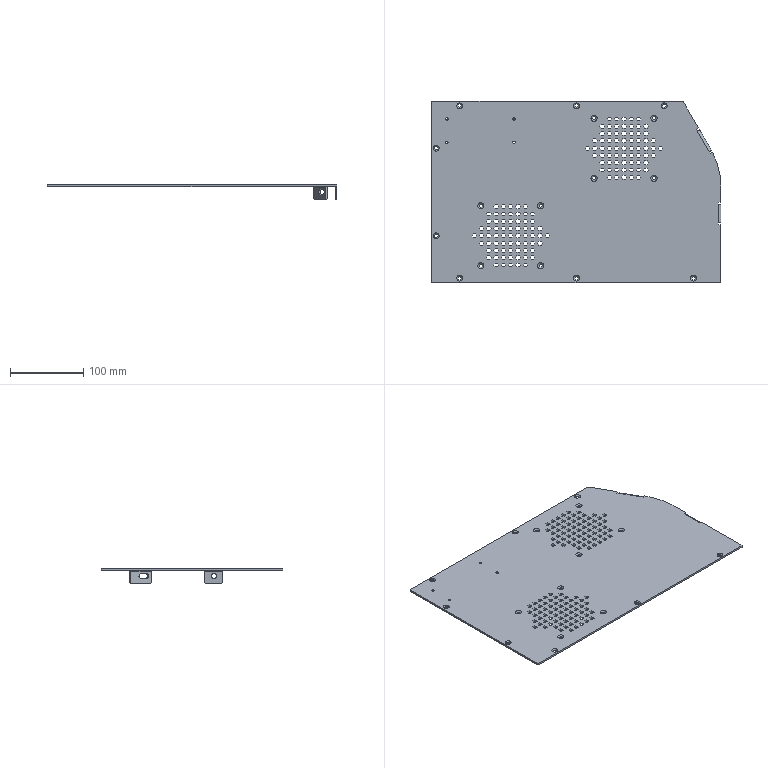Part | STEP file | AP0_ASM_JYDM_SHEET_04 | 1 solid | 926 faces | box 396.5 x 248 x 20 mm | volume 232744 mm3 | plane 844 | cylinder 50 | cone 32 | commonest cylinder face diameters 4.5 x16 5 x16 3.3 x8 7 x6 1.6 x1 2 x1